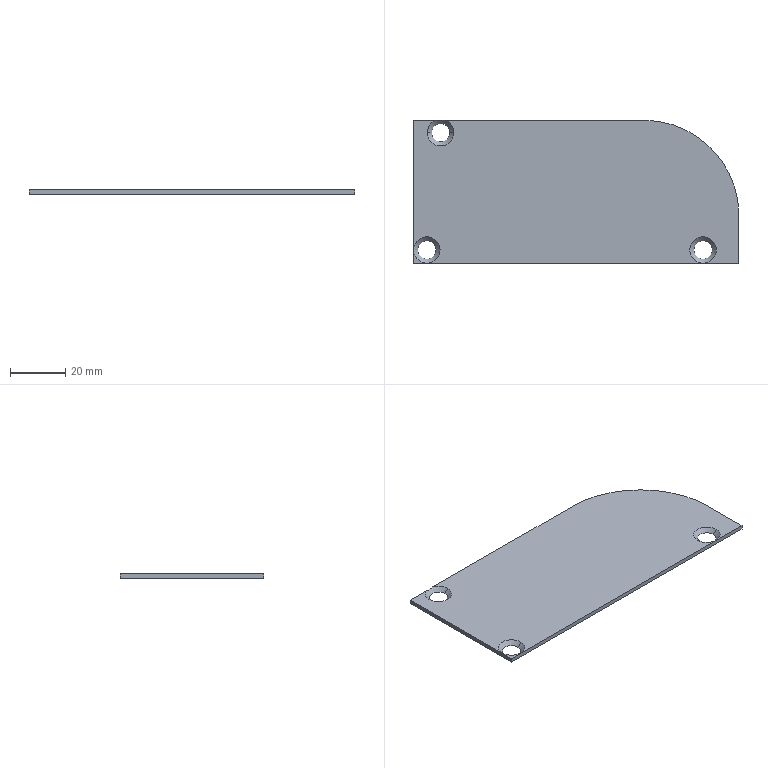Part | STEP file | 601-01-0001 | 1 solid | 13 faces | box 118 x 52 x 1.5 mm | volume 8586 mm3 | cone 6 | plane 6 | cylinder 1 | commonest cylinder face diameters 69 x1
STEP:
#1=CARTESIAN_POINT('',(0.,0.,0.));
#2=DIRECTION('',(0.,0.,1.));
#3=DIRECTION('',(1.,0.,0.));
#4=AXIS2_PLACEMENT_3D('',#1,#2,#3);
#5=CARTESIAN_POINT('',(-45.7,21.5,0.));
#6=VERTEX_POINT('',#5);
#7=CARTESIAN_POINT('',(-44.2,21.5,1.5));
#8=VERTEX_POINT('',#7);
#9=CARTESIAN_POINT('',(-44.2,21.5,1.5));
#10=DIRECTION('',(0.7071,0.,0.7071));
#11=VECTOR('',#10,1.);
#12=LINE('',#9,#11);
#13=CARTESIAN_POINT('',(-49.,21.5,1.5));
#14=DIRECTION('',(0.,0.,1.));
#15=DIRECTION('',(1.,0.,0.));
#16=AXIS2_PLACEMENT_3D('',#13,#14,#15);
#17=CONICAL_SURFACE('',#16,4.8,0.7854);
#18=CARTESIAN_POINT('',(6.283,0.));
#19=DIRECTION('',(0.,1.));
#20=VECTOR('',#19,1.);
#21=LINE('',#18,#20);
#22=(GEOMETRIC_REPRESENTATION_CONTEXT(2)PARAMETRIC_REPRESENTATION_CONTEXT()REPRESENTATION_CONTEXT('',''));
#23=DEFINITIONAL_REPRESENTATION('',(#21),#22);
#24=PCURVE('',#17,#23);
#25=CARTESIAN_POINT('',(-49.,21.5,1.5));
#26=DIRECTION('',(0.,0.,1.));
#27=DIRECTION('',(1.,0.,0.));
#28=AXIS2_PLACEMENT_3D('',#25,#26,#27);
#29=CONICAL_SURFACE('',#28,4.8,0.7854);
#30=CARTESIAN_POINT('',(0.,0.));
#31=DIRECTION('',(0.,1.));
#32=VECTOR('',#31,1.);
#33=LINE('',#30,#32);
#34=(GEOMETRIC_REPRESENTATION_CONTEXT(2)PARAMETRIC_REPRESENTATION_CONTEXT()REPRESENTATION_CONTEXT('',''));
#35=DEFINITIONAL_REPRESENTATION('',(#33),#34);
#36=PCURVE('',#29,#35);
#37=SURFACE_CURVE('',#12,(#24,#36),.PCURVE_S1.);
#38=EDGE_CURVE('',#6,#8,#37,.T.);
#39=ORIENTED_EDGE('',*,*,#38,.T.);
#40=CARTESIAN_POINT('',(-53.8,21.5,1.5));
#41=VERTEX_POINT('',#40);
#42=CARTESIAN_POINT('',(-49.,21.5,1.5));
#43=DIRECTION('',(0.,0.,1.));
#44=DIRECTION('',(1.,0.,0.));
#45=AXIS2_PLACEMENT_3D('',#42,#43,#44);
#46=CIRCLE('',#45,4.8);
#47=CARTESIAN_POINT('',(0.,0.));
#48=DIRECTION('',(1.,0.));
#49=VECTOR('',#48,1.);
#50=LINE('',#47,#49);
#51=(GEOMETRIC_REPRESENTATION_CONTEXT(2)PARAMETRIC_REPRESENTATION_CONTEXT()REPRESENTATION_CONTEXT('',''));
#52=DEFINITIONAL_REPRESENTATION('',(#50),#51);
#53=PCURVE('',#17,#52);
#54=CARTESIAN_POINT('',(59.,-26.,1.5));
#55=DIRECTION('',(0.,0.,1.));
#56=DIRECTION('',(1.,0.,0.));
#57=AXIS2_PLACEMENT_3D('',#54,#55,#56);
#58=PLANE('',#57);
#59=CARTESIAN_POINT('',(-108.,47.5));
#60=DIRECTION('',(1.,0.));
#61=AXIS2_PLACEMENT_2D('',#59,#60);
#62=CIRCLE('',#61,4.8);
#63=(GEOMETRIC_REPRESENTATION_CONTEXT(2)PARAMETRIC_REPRESENTATION_CONTEXT()REPRESENTATION_CONTEXT('',''));
#64=DEFINITIONAL_REPRESENTATION('',(#62),#63);
#65=PCURVE('',#58,#64);
#66=SURFACE_CURVE('',#46,(#53,#65),.PCURVE_S1.);
#67=EDGE_CURVE('',#41,#8,#66,.T.);
#68=ORIENTED_EDGE('',*,*,#67,.F.);
#69=CARTESIAN_POINT('',(-52.3,21.5,0.));
#70=VERTEX_POINT('',#69);
#71=CARTESIAN_POINT('',(-53.8,21.5,1.5));
#72=DIRECTION('',(-0.7071,0.,0.7071));
#73=VECTOR('',#72,1.);
#74=LINE('',#71,#73);
#75=CARTESIAN_POINT('',(3.142,0.));
#76=DIRECTION('',(0.,1.));
#77=VECTOR('',#76,1.);
#78=LINE('',#75,#77);
#79=(GEOMETRIC_REPRESENTATION_CONTEXT(2)PARAMETRIC_REPRESENTATION_CONTEXT()REPRESENTATION_CONTEXT('',''));
#80=DEFINITIONAL_REPRESENTATION('',(#78),#79);
#81=PCURVE('',#17,#80);
#82=CARTESIAN_POINT('',(3.142,0.));
#83=DIRECTION('',(0.,1.));
#84=VECTOR('',#83,1.);
#85=LINE('',#82,#84);
#86=(GEOMETRIC_REPRESENTATION_CONTEXT(2)PARAMETRIC_REPRESENTATION_CONTEXT()REPRESENTATION_CONTEXT('',''));
#87=DEFINITIONAL_REPRESENTATION('',(#85),#86);
#88=PCURVE('',#29,#87);
#89=SURFACE_CURVE('',#74,(#81,#88),.PCURVE_S1.);
#90=EDGE_CURVE('',#70,#41,#89,.T.);
#91=ORIENTED_EDGE('',*,*,#90,.F.);
#92=CARTESIAN_POINT('',(-49.,21.5,0.));
#93=DIRECTION('',(0.,0.,1.));
#94=DIRECTION('',(1.,0.,0.));
#95=AXIS2_PLACEMENT_3D('',#92,#93,#94);
#96=CIRCLE('',#95,3.3);
#97=CARTESIAN_POINT('',(0.,-1.5));
#98=DIRECTION('',(1.,0.));
#99=VECTOR('',#98,1.);
#100=LINE('',#97,#99);
#101=(GEOMETRIC_REPRESENTATION_CONTEXT(2)PARAMETRIC_REPRESENTATION_CONTEXT()REPRESENTATION_CONTEXT('',''));
#102=DEFINITIONAL_REPRESENTATION('',(#100),#101);
#103=PCURVE('',#17,#102);
#104=CARTESIAN_POINT('',(59.,-26.,0.));
#105=DIRECTION('',(0.,0.,1.));
#106=DIRECTION('',(1.,0.,0.));
#107=AXIS2_PLACEMENT_3D('',#104,#105,#106);
#108=PLANE('',#107);
#109=CARTESIAN_POINT('',(-108.,47.5));
#110=DIRECTION('',(1.,0.));
#111=AXIS2_PLACEMENT_2D('',#109,#110);
#112=CIRCLE('',#111,3.3);
#113=(GEOMETRIC_REPRESENTATION_CONTEXT(2)PARAMETRIC_REPRESENTATION_CONTEXT()REPRESENTATION_CONTEXT('',''));
#114=DEFINITIONAL_REPRESENTATION('',(#112),#113);
#115=PCURVE('',#108,#114);
#116=SURFACE_CURVE('',#96,(#103,#115),.PCURVE_S1.);
#117=EDGE_CURVE('',#70,#6,#116,.T.);
#118=ORIENTED_EDGE('',*,*,#117,.T.);
#119=EDGE_LOOP('',(#39,#68,#91,#118));
#120=FACE_BOUND('',#119,.F.);
#121=ADVANCED_FACE('',(#120),#17,.F.);
#122=CARTESIAN_POINT('',(-50.7,-21.,0.));
#123=VERTEX_POINT('',#122);
#124=CARTESIAN_POINT('',(-49.2,-21.,1.5));
#125=VERTEX_POINT('',#124);
#126=CARTESIAN_POINT('',(-49.2,-21.,1.5));
#127=DIRECTION('',(0.7071,0.,0.7071));
#128=VECTOR('',#127,1.);
#129=LINE('',#126,#128);
#130=CARTESIAN_POINT('',(-54.,-21.,1.5));
#131=DIRECTION('',(0.,0.,1.));
#132=DIRECTION('',(1.,0.,0.));
#133=AXIS2_PLACEMENT_3D('',#130,#131,#132);
#134=CONICAL_SURFACE('',#133,4.8,0.7854);
#135=CARTESIAN_POINT('',(6.283,0.));
#136=DIRECTION('',(0.,1.));
#137=VECTOR('',#136,1.);
#138=LINE('',#135,#137);
#139=(GEOMETRIC_REPRESENTATION_CONTEXT(2)PARAMETRIC_REPRESENTATION_CONTEXT()REPRESENTATION_CONTEXT('',''));
#140=DEFINITIONAL_REPRESENTATION('',(#138),#139);
#141=PCURVE('',#134,#140);
#142=CARTESIAN_POINT('',(-54.,-21.,1.5));
#143=DIRECTION('',(0.,0.,1.));
#144=DIRECTION('',(1.,0.,0.));
#145=AXIS2_PLACEMENT_3D('',#142,#143,#144);
#146=CONICAL_SURFACE('',#145,4.8,0.7854);
#147=CARTESIAN_POINT('',(0.,0.));
#148=DIRECTION('',(0.,1.));
#149=VECTOR('',#148,1.);
#150=LINE('',#147,#149);
#151=(GEOMETRIC_REPRESENTATION_CONTEXT(2)PARAMETRIC_REPRESENTATION_CONTEXT()REPRESENTATION_CONTEXT('',''));
#152=DEFINITIONAL_REPRESENTATION('',(#150),#151);
#153=PCURVE('',#146,#152);
#154=SURFACE_CURVE('',#129,(#141,#153),.PCURVE_S1.);
#155=EDGE_CURVE('',#123,#125,#154,.T.);
#156=ORIENTED_EDGE('',*,*,#155,.T.);
#157=CARTESIAN_POINT('',(-58.8,-21.,1.5));
#158=VERTEX_POINT('',#157);
#159=CARTESIAN_POINT('',(-54.,-21.,1.5));
#160=DIRECTION('',(0.,0.,1.));
#161=DIRECTION('',(1.,0.,0.));
#162=AXIS2_PLACEMENT_3D('',#159,#160,#161);
#163=CIRCLE('',#162,4.8);
#164=CARTESIAN_POINT('',(0.,0.));
#165=DIRECTION('',(1.,0.));
#166=VECTOR('',#165,1.);
#167=LINE('',#164,#166);
#168=(GEOMETRIC_REPRESENTATION_CONTEXT(2)PARAMETRIC_REPRESENTATION_CONTEXT()REPRESENTATION_CONTEXT('',''));
#169=DEFINITIONAL_REPRESENTATION('',(#167),#168);
#170=PCURVE('',#134,#169);
#171=CARTESIAN_POINT('',(-113.,5.));
#172=DIRECTION('',(1.,0.));
#173=AXIS2_PLACEMENT_2D('',#171,#172);
#174=CIRCLE('',#173,4.8);
#175=(GEOMETRIC_REPRESENTATION_CONTEXT(2)PARAMETRIC_REPRESENTATION_CONTEXT()REPRESENTATION_CONTEXT('',''));
#176=DEFINITIONAL_REPRESENTATION('',(#174),#175);
#177=PCURVE('',#58,#176);
#178=SURFACE_CURVE('',#163,(#170,#177),.PCURVE_S1.);
#179=EDGE_CURVE('',#158,#125,#178,.T.);
#180=ORIENTED_EDGE('',*,*,#179,.F.);
#181=CARTESIAN_POINT('',(-57.3,-21.,0.));
#182=VERTEX_POINT('',#181);
#183=CARTESIAN_POINT('',(-58.8,-21.,1.5));
#184=DIRECTION('',(-0.7071,0.,0.7071));
#185=VECTOR('',#184,1.);
#186=LINE('',#183,#185);
#187=CARTESIAN_POINT('',(3.142,0.));
#188=DIRECTION('',(0.,1.));
#189=VECTOR('',#188,1.);
#190=LINE('',#187,#189);
#191=(GEOMETRIC_REPRESENTATION_CONTEXT(2)PARAMETRIC_REPRESENTATION_CONTEXT()REPRESENTATION_CONTEXT('',''));
#192=DEFINITIONAL_REPRESENTATION('',(#190),#191);
#193=PCURVE('',#134,#192);
#194=CARTESIAN_POINT('',(3.142,0.));
#195=DIRECTION('',(0.,1.));
#196=VECTOR('',#195,1.);
#197=LINE('',#194,#196);
#198=(GEOMETRIC_REPRESENTATION_CONTEXT(2)PARAMETRIC_REPRESENTATION_CONTEXT()REPRESENTATION_CONTEXT('',''));
#199=DEFINITIONAL_REPRESENTATION('',(#197),#198);
#200=PCURVE('',#146,#199);
#201=SURFACE_CURVE('',#186,(#193,#200),.PCURVE_S1.);
#202=EDGE_CURVE('',#182,#158,#201,.T.);
#203=ORIENTED_EDGE('',*,*,#202,.F.);
#204=CARTESIAN_POINT('',(-54.,-21.,0.));
#205=DIRECTION('',(0.,0.,1.));
#206=DIRECTION('',(1.,0.,0.));
#207=AXIS2_PLACEMENT_3D('',#204,#205,#206);
#208=CIRCLE('',#207,3.3);
#209=CARTESIAN_POINT('',(0.,-1.5));
#210=DIRECTION('',(1.,0.));
#211=VECTOR('',#210,1.);
#212=LINE('',#209,#211);
#213=(GEOMETRIC_REPRESENTATION_CONTEXT(2)PARAMETRIC_REPRESENTATION_CONTEXT()REPRESENTATION_CONTEXT('',''));
#214=DEFINITIONAL_REPRESENTATION('',(#212),#213);
#215=PCURVE('',#134,#214);
#216=CARTESIAN_POINT('',(-113.,5.));
#217=DIRECTION('',(1.,0.));
#218=AXIS2_PLACEMENT_2D('',#216,#217);
#219=CIRCLE('',#218,3.3);
#220=(GEOMETRIC_REPRESENTATION_CONTEXT(2)PARAMETRIC_REPRESENTATION_CONTEXT()REPRESENTATION_CONTEXT('',''));
#221=DEFINITIONAL_REPRESENTATION('',(#219),#220);
#222=PCURVE('',#108,#221);
#223=SURFACE_CURVE('',#208,(#215,#222),.PCURVE_S1.);
#224=EDGE_CURVE('',#182,#123,#223,.T.);
#225=ORIENTED_EDGE('',*,*,#224,.T.);
#226=EDGE_LOOP('',(#156,#180,#203,#225));
#227=FACE_BOUND('',#226,.F.);
#228=ADVANCED_FACE('',(#227),#134,.F.);
#229=CARTESIAN_POINT('',(49.3,-21.,0.));
#230=VERTEX_POINT('',#229);
#231=CARTESIAN_POINT('',(50.8,-21.,1.5));
#232=VERTEX_POINT('',#231);
#233=CARTESIAN_POINT('',(50.8,-21.,1.5));
#234=DIRECTION('',(0.7071,0.,0.7071));
#235=VECTOR('',#234,1.);
#236=LINE('',#233,#235);
#237=CARTESIAN_POINT('',(46.,-21.,1.5));
#238=DIRECTION('',(0.,0.,1.));
#239=DIRECTION('',(1.,0.,0.));
#240=AXIS2_PLACEMENT_3D('',#237,#238,#239);
#241=CONICAL_SURFACE('',#240,4.8,0.7854);
#242=CARTESIAN_POINT('',(6.283,0.));
#243=DIRECTION('',(0.,1.));
#244=VECTOR('',#243,1.);
#245=LINE('',#242,#244);
#246=(GEOMETRIC_REPRESENTATION_CONTEXT(2)PARAMETRIC_REPRESENTATION_CONTEXT()REPRESENTATION_CONTEXT('',''));
#247=DEFINITIONAL_REPRESENTATION('',(#245),#246);
#248=PCURVE('',#241,#247);
#249=CARTESIAN_POINT('',(46.,-21.,1.5));
#250=DIRECTION('',(0.,0.,1.));
#251=DIRECTION('',(1.,0.,0.));
#252=AXIS2_PLACEMENT_3D('',#249,#250,#251);
#253=CONICAL_SURFACE('',#252,4.8,0.7854);
#254=CARTESIAN_POINT('',(0.,0.));
#255=DIRECTION('',(0.,1.));
#256=VECTOR('',#255,1.);
#257=LINE('',#254,#256);
#258=(GEOMETRIC_REPRESENTATION_CONTEXT(2)PARAMETRIC_REPRESENTATION_CONTEXT()REPRESENTATION_CONTEXT('',''));
#259=DEFINITIONAL_REPRESENTATION('',(#257),#258);
#260=PCURVE('',#253,#259);
#261=SURFACE_CURVE('',#236,(#248,#260),.PCURVE_S1.);
#262=EDGE_CURVE('',#230,#232,#261,.T.);
#263=ORIENTED_EDGE('',*,*,#262,.T.);
#264=CARTESIAN_POINT('',(41.2,-21.,1.5));
#265=VERTEX_POINT('',#264);
#266=CARTESIAN_POINT('',(46.,-21.,1.5));
#267=DIRECTION('',(0.,0.,1.));
#268=DIRECTION('',(1.,0.,0.));
#269=AXIS2_PLACEMENT_3D('',#266,#267,#268);
#270=CIRCLE('',#269,4.8);
#271=CARTESIAN_POINT('',(0.,0.));
#272=DIRECTION('',(1.,0.));
#273=VECTOR('',#272,1.);
#274=LINE('',#271,#273);
#275=(GEOMETRIC_REPRESENTATION_CONTEXT(2)PARAMETRIC_REPRESENTATION_CONTEXT()REPRESENTATION_CONTEXT('',''));
#276=DEFINITIONAL_REPRESENTATION('',(#274),#275);
#277=PCURVE('',#241,#276);
#278=CARTESIAN_POINT('',(-13.,5.));
#279=DIRECTION('',(1.,0.));
#280=AXIS2_PLACEMENT_2D('',#278,#279);
#281=CIRCLE('',#280,4.8);
#282=(GEOMETRIC_REPRESENTATION_CONTEXT(2)PARAMETRIC_REPRESENTATION_CONTEXT()REPRESENTATION_CONTEXT('',''));
#283=DEFINITIONAL_REPRESENTATION('',(#281),#282);
#284=PCURVE('',#58,#283);
#285=SURFACE_CURVE('',#270,(#277,#284),.PCURVE_S1.);
#286=EDGE_CURVE('',#265,#232,#285,.T.);
#287=ORIENTED_EDGE('',*,*,#286,.F.);
#288=CARTESIAN_POINT('',(42.7,-21.,0.));
#289=VERTEX_POINT('',#288);
#290=CARTESIAN_POINT('',(41.2,-21.,1.5));
#291=DIRECTION('',(-0.7071,0.,0.7071));
#292=VECTOR('',#291,1.);
#293=LINE('',#290,#292);
#294=CARTESIAN_POINT('',(3.142,0.));
#295=DIRECTION('',(0.,1.));
#296=VECTOR('',#295,1.);
#297=LINE('',#294,#296);
#298=(GEOMETRIC_REPRESENTATION_CONTEXT(2)PARAMETRIC_REPRESENTATION_CONTEXT()REPRESENTATION_CONTEXT('',''));
#299=DEFINITIONAL_REPRESENTATION('',(#297),#298);
#300=PCURVE('',#241,#299);
#301=CARTESIAN_POINT('',(3.142,0.));
#302=DIRECTION('',(0.,1.));
#303=VECTOR('',#302,1.);
#304=LINE('',#301,#303);
#305=(GEOMETRIC_REPRESENTATION_CONTEXT(2)PARAMETRIC_REPRESENTATION_CONTEXT()REPRESENTATION_CONTEXT('',''));
#306=DEFINITIONAL_REPRESENTATION('',(#304),#305);
#307=PCURVE('',#253,#306);
#308=SURFACE_CURVE('',#293,(#300,#307),.PCURVE_S1.);
#309=EDGE_CURVE('',#289,#265,#308,.T.);
#310=ORIENTED_EDGE('',*,*,#309,.F.);
#311=CARTESIAN_POINT('',(46.,-21.,0.));
#312=DIRECTION('',(0.,0.,1.));
#313=DIRECTION('',(1.,0.,0.));
#314=AXIS2_PLACEMENT_3D('',#311,#312,#313);
#315=CIRCLE('',#314,3.3);
#316=CARTESIAN_POINT('',(0.,-1.5));
#317=DIRECTION('',(1.,0.));
#318=VECTOR('',#317,1.);
#319=LINE('',#316,#318);
#320=(GEOMETRIC_REPRESENTATION_CONTEXT(2)PARAMETRIC_REPRESENTATION_CONTEXT()REPRESENTATION_CONTEXT('',''));
#321=DEFINITIONAL_REPRESENTATION('',(#319),#320);
#322=PCURVE('',#241,#321);
#323=CARTESIAN_POINT('',(-13.,5.));
#324=DIRECTION('',(1.,0.));
#325=AXIS2_PLACEMENT_2D('',#323,#324);
#326=CIRCLE('',#325,3.3);
#327=(GEOMETRIC_REPRESENTATION_CONTEXT(2)PARAMETRIC_REPRESENTATION_CONTEXT()REPRESENTATION_CONTEXT('',''));
#328=DEFINITIONAL_REPRESENTATION('',(#326),#327);
#329=PCURVE('',#108,#328);
#330=SURFACE_CURVE('',#315,(#322,#329),.PCURVE_S1.);
#331=EDGE_CURVE('',#289,#230,#330,.T.);
#332=ORIENTED_EDGE('',*,*,#331,.T.);
#333=EDGE_LOOP('',(#263,#287,#310,#332));
#334=FACE_BOUND('',#333,.F.);
#335=ADVANCED_FACE('',(#334),#241,.F.);
#336=CARTESIAN_POINT('',(-49.,21.5,0.));
#337=DIRECTION('',(0.,0.,1.));
#338=DIRECTION('',(1.,0.,0.));
#339=AXIS2_PLACEMENT_3D('',#336,#337,#338);
#340=CIRCLE('',#339,3.3);
#341=CARTESIAN_POINT('',(-108.,47.5));
#342=DIRECTION('',(1.,0.));
#343=AXIS2_PLACEMENT_2D('',#341,#342);
#344=CIRCLE('',#343,3.3);
#345=(GEOMETRIC_REPRESENTATION_CONTEXT(2)PARAMETRIC_REPRESENTATION_CONTEXT()REPRESENTATION_CONTEXT('',''));
#346=DEFINITIONAL_REPRESENTATION('',(#344),#345);
#347=PCURVE('',#108,#346);
#348=CARTESIAN_POINT('',(0.,-1.5));
#349=DIRECTION('',(1.,0.));
#350=VECTOR('',#349,1.);
#351=LINE('',#348,#350);
#352=(GEOMETRIC_REPRESENTATION_CONTEXT(2)PARAMETRIC_REPRESENTATION_CONTEXT()REPRESENTATION_CONTEXT('',''));
#353=DEFINITIONAL_REPRESENTATION('',(#351),#352);
#354=PCURVE('',#29,#353);
#355=SURFACE_CURVE('',#340,(#347,#354),.PCURVE_S1.);
#356=EDGE_CURVE('',#6,#70,#355,.T.);
#357=ORIENTED_EDGE('',*,*,#356,.T.);
#358=ORIENTED_EDGE('',*,*,#117,.T.);
#359=EDGE_LOOP('',(#357,#358));
#360=FACE_BOUND('',#359,.T.);
#361=CARTESIAN_POINT('',(-54.,-21.,0.));
#362=DIRECTION('',(0.,0.,1.));
#363=DIRECTION('',(1.,0.,0.));
#364=AXIS2_PLACEMENT_3D('',#361,#362,#363);
#365=CIRCLE('',#364,3.3);
#366=CARTESIAN_POINT('',(-113.,5.));
#367=DIRECTION('',(1.,0.));
#368=AXIS2_PLACEMENT_2D('',#366,#367);
#369=CIRCLE('',#368,3.3);
#370=(GEOMETRIC_REPRESENTATION_CONTEXT(2)PARAMETRIC_REPRESENTATION_CONTEXT()REPRESENTATION_CONTEXT('',''));
#371=DEFINITIONAL_REPRESENTATION('',(#369),#370);
#372=PCURVE('',#108,#371);
#373=CARTESIAN_POINT('',(0.,-1.5));
#374=DIRECTION('',(1.,0.));
#375=VECTOR('',#374,1.);
#376=LINE('',#373,#375);
#377=(GEOMETRIC_REPRESENTATION_CONTEXT(2)PARAMETRIC_REPRESENTATION_CONTEXT()REPRESENTATION_CONTEXT('',''));
#378=DEFINITIONAL_REPRESENTATION('',(#376),#377);
#379=PCURVE('',#146,#378);
#380=SURFACE_CURVE('',#365,(#372,#379),.PCURVE_S1.);
#381=EDGE_CURVE('',#123,#182,#380,.T.);
#382=ORIENTED_EDGE('',*,*,#381,.T.);
#383=ORIENTED_EDGE('',*,*,#224,.T.);
#384=EDGE_LOOP('',(#382,#383));
#385=FACE_BOUND('',#384,.T.);
#386=CARTESIAN_POINT('',(24.5,26.,0.));
#387=VERTEX_POINT('',#386);
#388=CARTESIAN_POINT('',(-59.,26.,0.));
#389=VERTEX_POINT('',#388);
#390=CARTESIAN_POINT('',(-59.,26.,0.));
#391=DIRECTION('',(-1.,0.,0.));
#392=VECTOR('',#391,1.);
#393=LINE('',#390,#392);
#394=CARTESIAN_POINT('',(-118.,52.));
#395=DIRECTION('',(-1.,0.));
#396=VECTOR('',#395,1.);
#397=LINE('',#394,#396);
#398=(GEOMETRIC_REPRESENTATION_CONTEXT(2)PARAMETRIC_REPRESENTATION_CONTEXT()REPRESENTATION_CONTEXT('',''));
#399=DEFINITIONAL_REPRESENTATION('',(#397),#398);
#400=PCURVE('',#108,#399);
#401=CARTESIAN_POINT('',(-59.,26.,1.5));
#402=DIRECTION('',(0.,-1.,0.));
#403=DIRECTION('',(0.,0.,-1.));
#404=AXIS2_PLACEMENT_3D('',#401,#402,#403);
#405=PLANE('',#404);
#406=CARTESIAN_POINT('',(1.5,0.));
#407=DIRECTION('',(0.,-1.));
#408=VECTOR('',#407,1.);
#409=LINE('',#406,#408);
#410=(GEOMETRIC_REPRESENTATION_CONTEXT(2)PARAMETRIC_REPRESENTATION_CONTEXT()REPRESENTATION_CONTEXT('',''));
#411=DEFINITIONAL_REPRESENTATION('',(#409),#410);
#412=PCURVE('',#405,#411);
#413=SURFACE_CURVE('',#393,(#400,#412),.PCURVE_S1.);
#414=EDGE_CURVE('',#387,#389,#413,.T.);
#415=ORIENTED_EDGE('',*,*,#414,.F.);
#416=CARTESIAN_POINT('',(59.,-8.5,0.));
#417=VERTEX_POINT('',#416);
#418=CARTESIAN_POINT('',(24.5,-8.5,0.));
#419=DIRECTION('',(0.,0.,-1.));
#420=DIRECTION('',(1.,0.,0.));
#421=AXIS2_PLACEMENT_3D('',#418,#419,#420);
#422=CIRCLE('',#421,34.5);
#423=CARTESIAN_POINT('',(0.,17.5));
#424=CARTESIAN_POINT('',(0.,-42.256));
#425=CARTESIAN_POINT('',(-51.75,-12.378));
#426=CARTESIAN_POINT('',(-103.5,17.5));
#427=CARTESIAN_POINT('',(-51.75,47.378));
#428=CARTESIAN_POINT('',(0.,77.256));
#429=CARTESIAN_POINT('',(0.,17.5));
#430=(BOUNDED_CURVE()B_SPLINE_CURVE(2,(#423,#424,#425,#426,#427,#428,#429),.UNSPECIFIED.,.T.,.F.)B_SPLINE_CURVE_WITH_KNOTS((1,2,2,2,2,1),(-2.094,0.,2.094,4.189,6.283,8.378),.UNSPECIFIED.)CURVE()GEOMETRIC_REPRESENTATION_ITEM()RATIONAL_B_SPLINE_CURVE((1.,0.5,1.,0.5,1.,0.5,1.))REPRESENTATION_ITEM(''));
#431=(GEOMETRIC_REPRESENTATION_CONTEXT(2)PARAMETRIC_REPRESENTATION_CONTEXT()REPRESENTATION_CONTEXT('',''));
#432=DEFINITIONAL_REPRESENTATION('',(#430),#431);
#433=PCURVE('',#108,#432);
#434=CARTESIAN_POINT('',(24.5,-8.5,1.5));
#435=DIRECTION('',(0.,0.,-1.));
#436=DIRECTION('',(-1.,0.,0.));
#437=AXIS2_PLACEMENT_3D('',#434,#435,#436);
#438=CYLINDRICAL_SURFACE('',#437,34.5);
#439=CARTESIAN_POINT('',(-3.142,1.5));
#440=DIRECTION('',(1.,0.));
#441=VECTOR('',#440,1.);
#442=LINE('',#439,#441);
#443=(GEOMETRIC_REPRESENTATION_CONTEXT(2)PARAMETRIC_REPRESENTATION_CONTEXT()REPRESENTATION_CONTEXT('',''));
#444=DEFINITIONAL_REPRESENTATION('',(#442),#443);
#445=PCURVE('',#438,#444);
#446=SURFACE_CURVE('',#422,(#433,#445),.PCURVE_S1.);
#447=EDGE_CURVE('',#387,#417,#446,.T.);
#448=ORIENTED_EDGE('',*,*,#447,.T.);
#449=CARTESIAN_POINT('',(59.,-26.,0.));
#450=VERTEX_POINT('',#449);
#451=CARTESIAN_POINT('',(59.,26.,0.));
#452=DIRECTION('',(0.,1.,0.));
#453=VECTOR('',#452,1.);
#454=LINE('',#451,#453);
#455=CARTESIAN_POINT('',(0.,52.));
#456=DIRECTION('',(0.,1.));
#457=VECTOR('',#456,1.);
#458=LINE('',#455,#457);
#459=(GEOMETRIC_REPRESENTATION_CONTEXT(2)PARAMETRIC_REPRESENTATION_CONTEXT()REPRESENTATION_CONTEXT('',''));
#460=DEFINITIONAL_REPRESENTATION('',(#458),#459);
#461=PCURVE('',#108,#460);
#462=CARTESIAN_POINT('',(59.,26.,1.5));
#463=DIRECTION('',(-1.,0.,0.));
#464=DIRECTION('',(0.,-1.,0.));
#465=AXIS2_PLACEMENT_3D('',#462,#463,#464);
#466=PLANE('',#465);
#467=CARTESIAN_POINT('',(0.,-1.5));
#468=DIRECTION('',(-1.,0.));
#469=VECTOR('',#468,1.);
#470=LINE('',#467,#469);
#471=(GEOMETRIC_REPRESENTATION_CONTEXT(2)PARAMETRIC_REPRESENTATION_CONTEXT()REPRESENTATION_CONTEXT('',''));
#472=DEFINITIONAL_REPRESENTATION('',(#470),#471);
#473=PCURVE('',#466,#472);
#474=SURFACE_CURVE('',#454,(#461,#473),.PCURVE_S1.);
#475=EDGE_CURVE('',#450,#417,#474,.T.);
#476=ORIENTED_EDGE('',*,*,#475,.F.);
#477=CARTESIAN_POINT('',(-59.,-26.,0.));
#478=VERTEX_POINT('',#477);
#479=CARTESIAN_POINT('',(-59.,-26.,0.));
#480=DIRECTION('',(1.,0.,0.));
#481=VECTOR('',#480,1.);
#482=LINE('',#479,#481);
#483=CARTESIAN_POINT('',(-118.,0.));
#484=DIRECTION('',(1.,0.));
#485=VECTOR('',#484,1.);
#486=LINE('',#483,#485);
#487=(GEOMETRIC_REPRESENTATION_CONTEXT(2)PARAMETRIC_REPRESENTATION_CONTEXT()REPRESENTATION_CONTEXT('',''));
#488=DEFINITIONAL_REPRESENTATION('',(#486),#487);
#489=PCURVE('',#108,#488);
#490=CARTESIAN_POINT('',(-59.,-26.,1.5));
#491=DIRECTION('',(0.,1.,0.));
#492=DIRECTION('',(0.,0.,1.));
#493=AXIS2_PLACEMENT_3D('',#490,#491,#492);
#494=PLANE('',#493);
#495=CARTESIAN_POINT('',(-1.5,0.));
#496=DIRECTION('',(0.,1.));
#497=VECTOR('',#496,1.);
#498=LINE('',#495,#497);
#499=(GEOMETRIC_REPRESENTATION_CONTEXT(2)PARAMETRIC_REPRESENTATION_CONTEXT()REPRESENTATION_CONTEXT('',''));
#500=DEFINITIONAL_REPRESENTATION('',(#498),#499);
#501=PCURVE('',#494,#500);
#502=SURFACE_CURVE('',#482,(#489,#501),.PCURVE_S1.);
#503=EDGE_CURVE('',#478,#450,#502,.T.);
#504=ORIENTED_EDGE('',*,*,#503,.F.);
#505=CARTESIAN_POINT('',(-59.,26.,0.));
#506=DIRECTION('',(0.,-1.,0.));
#507=VECTOR('',#506,1.);
#508=LINE('',#505,#507);
#509=CARTESIAN_POINT('',(-118.,52.));
#510=DIRECTION('',(0.,-1.));
#511=VECTOR('',#510,1.);
#512=LINE('',#509,#511);
#513=(GEOMETRIC_REPRESENTATION_CONTEXT(2)PARAMETRIC_REPRESENTATION_CONTEXT()REPRESENTATION_CONTEXT('',''));
#514=DEFINITIONAL_REPRESENTATION('',(#512),#513);
#515=PCURVE('',#108,#514);
#516=CARTESIAN_POINT('',(-59.,26.,1.5));
#517=DIRECTION('',(1.,0.,0.));
#518=DIRECTION('',(0.,1.,0.));
#519=AXIS2_PLACEMENT_3D('',#516,#517,#518);
#520=PLANE('',#519);
#521=CARTESIAN_POINT('',(0.,-1.5));
#522=DIRECTION('',(-1.,0.));
#523=VECTOR('',#522,1.);
#524=LINE('',#521,#523);
#525=(GEOMETRIC_REPRESENTATION_CONTEXT(2)PARAMETRIC_REPRESENTATION_CONTEXT()REPRESENTATION_CONTEXT('',''));
#526=DEFINITIONAL_REPRESENTATION('',(#524),#525);
#527=PCURVE('',#520,#526);
#528=SURFACE_CURVE('',#508,(#515,#527),.PCURVE_S1.);
#529=EDGE_CURVE('',#389,#478,#528,.T.);
#530=ORIENTED_EDGE('',*,*,#529,.F.);
#531=EDGE_LOOP('',(#415,#448,#476,#504,#530));
#532=FACE_BOUND('',#531,.T.);
#533=CARTESIAN_POINT('',(46.,-21.,0.));
#534=DIRECTION('',(0.,0.,1.));
#535=DIRECTION('',(1.,0.,0.));
#536=AXIS2_PLACEMENT_3D('',#533,#534,#535);
#537=CIRCLE('',#536,3.3);
#538=CARTESIAN_POINT('',(-13.,5.));
#539=DIRECTION('',(1.,0.));
#540=AXIS2_PLACEMENT_2D('',#538,#539);
#541=CIRCLE('',#540,3.3);
#542=(GEOMETRIC_REPRESENTATION_CONTEXT(2)PARAMETRIC_REPRESENTATION_CONTEXT()REPRESENTATION_CONTEXT('',''));
#543=DEFINITIONAL_REPRESENTATION('',(#541),#542);
#544=PCURVE('',#108,#543);
#545=CARTESIAN_POINT('',(0.,-1.5));
#546=DIRECTION('',(1.,0.));
#547=VECTOR('',#546,1.);
#548=LINE('',#545,#547);
#549=(GEOMETRIC_REPRESENTATION_CONTEXT(2)PARAMETRIC_REPRESENTATION_CONTEXT()REPRESENTATION_CONTEXT('',''));
#550=DEFINITIONAL_REPRESENTATION('',(#548),#549);
#551=PCURVE('',#253,#550);
#552=SURFACE_CURVE('',#537,(#544,#551),.PCURVE_S1.);
#553=EDGE_CURVE('',#230,#289,#552,.T.);
#554=ORIENTED_EDGE('',*,*,#553,.T.);
#555=ORIENTED_EDGE('',*,*,#331,.T.);
#556=EDGE_LOOP('',(#554,#555));
#557=FACE_BOUND('',#556,.T.);
#558=ADVANCED_FACE('',(#360,#385,#532,#557),#108,.F.);
#559=ORIENTED_EDGE('',*,*,#475,.T.);
#560=CARTESIAN_POINT('',(59.,-8.5,1.5));
#561=VERTEX_POINT('',#560);
#562=CARTESIAN_POINT('',(59.,-8.5,1.5));
#563=DIRECTION('',(0.,0.,1.));
#564=VECTOR('',#563,1.);
#565=LINE('',#562,#564);
#566=CARTESIAN_POINT('',(34.5,0.));
#567=DIRECTION('',(0.,1.));
#568=VECTOR('',#567,1.);
#569=LINE('',#566,#568);
#570=(GEOMETRIC_REPRESENTATION_CONTEXT(2)PARAMETRIC_REPRESENTATION_CONTEXT()REPRESENTATION_CONTEXT('',''));
#571=DEFINITIONAL_REPRESENTATION('',(#569),#570);
#572=PCURVE('',#466,#571);
#573=CARTESIAN_POINT('',(3.142,0.));
#574=DIRECTION('',(0.,-1.));
#575=VECTOR('',#574,1.);
#576=LINE('',#573,#575);
#577=(GEOMETRIC_REPRESENTATION_CONTEXT(2)PARAMETRIC_REPRESENTATION_CONTEXT()REPRESENTATION_CONTEXT('',''));
#578=DEFINITIONAL_REPRESENTATION('',(#576),#577);
#579=PCURVE('',#438,#578);
#580=SURFACE_CURVE('',#565,(#572,#579),.PCURVE_S1.);
#581=EDGE_CURVE('',#417,#561,#580,.T.);
#582=ORIENTED_EDGE('',*,*,#581,.T.);
#583=CARTESIAN_POINT('',(59.,-26.,1.5));
#584=VERTEX_POINT('',#583);
#585=CARTESIAN_POINT('',(59.,26.,1.5));
#586=DIRECTION('',(0.,1.,0.));
#587=VECTOR('',#586,1.);
#588=LINE('',#585,#587);
#589=CARTESIAN_POINT('',(0.,0.));
#590=DIRECTION('',(-1.,0.));
#591=VECTOR('',#590,1.);
#592=LINE('',#589,#591);
#593=(GEOMETRIC_REPRESENTATION_CONTEXT(2)PARAMETRIC_REPRESENTATION_CONTEXT()REPRESENTATION_CONTEXT('',''));
#594=DEFINITIONAL_REPRESENTATION('',(#592),#593);
#595=PCURVE('',#466,#594);
#596=CARTESIAN_POINT('',(0.,52.));
#597=DIRECTION('',(0.,1.));
#598=VECTOR('',#597,1.);
#599=LINE('',#596,#598);
#600=(GEOMETRIC_REPRESENTATION_CONTEXT(2)PARAMETRIC_REPRESENTATION_CONTEXT()REPRESENTATION_CONTEXT('',''));
#601=DEFINITIONAL_REPRESENTATION('',(#599),#600);
#602=PCURVE('',#58,#601);
#603=SURFACE_CURVE('',#588,(#595,#602),.PCURVE_S1.);
#604=EDGE_CURVE('',#584,#561,#603,.T.);
#605=ORIENTED_EDGE('',*,*,#604,.F.);
#606=CARTESIAN_POINT('',(59.,-26.,1.5));
#607=DIRECTION('',(0.,0.,-1.));
#608=VECTOR('',#607,1.);
#609=LINE('',#606,#608);
#610=CARTESIAN_POINT('',(52.,0.));
#611=DIRECTION('',(0.,-1.));
#612=VECTOR('',#611,1.);
#613=LINE('',#610,#612);
#614=(GEOMETRIC_REPRESENTATION_CONTEXT(2)PARAMETRIC_REPRESENTATION_CONTEXT()REPRESENTATION_CONTEXT('',''));
#615=DEFINITIONAL_REPRESENTATION('',(#613),#614);
#616=PCURVE('',#466,#615);
#617=CARTESIAN_POINT('',(0.,118.));
#618=DIRECTION('',(-1.,0.));
#619=VECTOR('',#618,1.);
#620=LINE('',#617,#619);
#621=(GEOMETRIC_REPRESENTATION_CONTEXT(2)PARAMETRIC_REPRESENTATION_CONTEXT()REPRESENTATION_CONTEXT('',''));
#622=DEFINITIONAL_REPRESENTATION('',(#620),#621);
#623=PCURVE('',#494,#622);
#624=SURFACE_CURVE('',#609,(#616,#623),.PCURVE_S1.);
#625=EDGE_CURVE('',#584,#450,#624,.T.);
#626=ORIENTED_EDGE('',*,*,#625,.T.);
#627=EDGE_LOOP('',(#559,#582,#605,#626));
#628=FACE_BOUND('',#627,.T.);
#629=ADVANCED_FACE('',(#628),#466,.F.);
#630=CARTESIAN_POINT('',(-50.67,26.,1.5));
#631=VERTEX_POINT('',#630);
#632=CARTESIAN_POINT('',(-59.,26.,1.5));
#633=VERTEX_POINT('',#632);
#634=CARTESIAN_POINT('',(-59.,26.,1.5));
#635=DIRECTION('',(-1.,0.,0.));
#636=VECTOR('',#635,1.);
#637=LINE('',#634,#636);
#638=CARTESIAN_POINT('',(0.,0.));
#639=DIRECTION('',(0.,-1.));
#640=VECTOR('',#639,1.);
#641=LINE('',#638,#640);
#642=(GEOMETRIC_REPRESENTATION_CONTEXT(2)PARAMETRIC_REPRESENTATION_CONTEXT()REPRESENTATION_CONTEXT('',''));
#643=DEFINITIONAL_REPRESENTATION('',(#641),#642);
#644=PCURVE('',#405,#643);
#645=CARTESIAN_POINT('',(-118.,52.));
#646=DIRECTION('',(-1.,0.));
#647=VECTOR('',#646,1.);
#648=LINE('',#645,#647);
#649=(GEOMETRIC_REPRESENTATION_CONTEXT(2)PARAMETRIC_REPRESENTATION_CONTEXT()REPRESENTATION_CONTEXT('',''));
#650=DEFINITIONAL_REPRESENTATION('',(#648),#649);
#651=PCURVE('',#58,#650);
#652=SURFACE_CURVE('',#637,(#644,#651),.PCURVE_S1.);
#653=EDGE_CURVE('',#631,#633,#652,.T.);
#654=ORIENTED_EDGE('',*,*,#653,.F.);
#655=CARTESIAN_POINT('',(-47.33,26.,1.5));
#656=VERTEX_POINT('',#655);
#657=CARTESIAN_POINT('',(-50.67,26.,1.5));
#658=CARTESIAN_POINT('',(-50.401,26.,1.406));
#659=CARTESIAN_POINT('',(-50.125,26.,1.33));
#660=CARTESIAN_POINT('',(-49.567,26.,1.227));
#661=CARTESIAN_POINT('',(-49.281,26.,1.2));
#662=CARTESIAN_POINT('',(-48.711,26.,1.2));
#663=CARTESIAN_POINT('',(-48.429,26.,1.228));
#664=CARTESIAN_POINT('',(-47.874,26.,1.331));
#665=CARTESIAN_POINT('',(-47.599,26.,1.406));
#666=CARTESIAN_POINT('',(-47.33,26.,1.5));
#667=B_SPLINE_CURVE_WITH_KNOTS('',3,(#657,#658,#659,#660,#661,#662,#663,#664,#665,#666),.UNSPECIFIED.,.F.,.F.,(4,2,2,2,4),(0.003213,0.004058,0.004902,0.005746,0.006591),.UNSPECIFIED.);
#668=CARTESIAN_POINT('',(0.,8.33));
#669=CARTESIAN_POINT('',(0.09372,8.599));
#670=CARTESIAN_POINT('',(0.1697,8.875));
#671=CARTESIAN_POINT('',(0.2728,9.433));
#672=CARTESIAN_POINT('',(0.3003,9.719));
#673=CARTESIAN_POINT('',(0.2997,10.289));
#674=CARTESIAN_POINT('',(0.2722,10.571));
#675=CARTESIAN_POINT('',(0.1694,11.126));
#676=CARTESIAN_POINT('',(0.0936,11.401));
#677=CARTESIAN_POINT('',(0.,11.67));
#678=B_SPLINE_CURVE_WITH_KNOTS('',3,(#668,#669,#670,#671,#672,#673,#674,#675,#676,#677),.UNSPECIFIED.,.F.,.F.,(4,2,2,2,4),(0.003213,0.004058,0.004902,0.005746,0.006591),.UNSPECIFIED.);
#679=(GEOMETRIC_REPRESENTATION_CONTEXT(2)PARAMETRIC_REPRESENTATION_CONTEXT()REPRESENTATION_CONTEXT('',''));
#680=DEFINITIONAL_REPRESENTATION('',(#678),#679);
#681=PCURVE('',#405,#680);
#682=CARTESIAN_POINT('',(1.926,0.));
#683=CARTESIAN_POINT('',(1.917,-0.01704));
#684=CARTESIAN_POINT('',(1.897,-0.04995));
#685=CARTESIAN_POINT('',(1.867,-0.09556));
#686=CARTESIAN_POINT('',(1.837,-0.1371));
#687=CARTESIAN_POINT('',(1.805,-0.1745));
#688=CARTESIAN_POINT('',(1.773,-0.2073));
#689=CARTESIAN_POINT('',(1.74,-0.2355));
#690=CARTESIAN_POINT('',(1.707,-0.2588));
#691=CARTESIAN_POINT('',(1.673,-0.2772));
#692=CARTESIAN_POINT('',(1.639,-0.2904));
#693=CARTESIAN_POINT('',(1.604,-0.2983));
#694=CARTESIAN_POINT('',(1.57,-0.3009));
#695=CARTESIAN_POINT('',(1.535,-0.298));
#696=CARTESIAN_POINT('',(1.501,-0.2899));
#697=CARTESIAN_POINT('',(1.467,-0.2766));
#698=CARTESIAN_POINT('',(1.434,-0.2583));
#699=CARTESIAN_POINT('',(1.401,-0.235));
#700=CARTESIAN_POINT('',(1.368,-0.2069));
#701=CARTESIAN_POINT('',(1.336,-0.1742));
#702=CARTESIAN_POINT('',(1.305,-0.1369));
#703=CARTESIAN_POINT('',(1.274,-0.09541));
#704=CARTESIAN_POINT('',(1.244,-0.04988));
#705=CARTESIAN_POINT('',(1.225,-0.01702));
#706=CARTESIAN_POINT('',(1.215,0.));
#707=B_SPLINE_CURVE_WITH_KNOTS('',3,(#682,#683,#684,#685,#686,#687,#688,#689,#690,#691,#692,#693,#694,#695,#696,#697,#698,#699,#700,#701,#702,#703,#704,#705,#706),.UNSPECIFIED.,.F.,.F.,(4,1,1,1,1,1,1,1,1,1,1,1,1,1,1,1,1,1,1,1,1,1,4),(0.003213,0.003367,0.00352,0.003674,0.003827,0.003981,0.004134,0.004288,0.004441,0.004595,0.004749,0.004902,0.005056,0.005209,0.005363,0.005516,0.00567,0.005823,0.005977,0.00613,0.006284,0.006437,0.006591),.QUASI_UNIFORM_KNOTS.);
#708=(GEOMETRIC_REPRESENTATION_CONTEXT(2)PARAMETRIC_REPRESENTATION_CONTEXT()REPRESENTATION_CONTEXT('',''));
#709=DEFINITIONAL_REPRESENTATION('',(#707),#708);
#710=PCURVE('',#29,#709);
#711=SURFACE_CURVE('',#667,(#681,#710),.PCURVE_S1.);
#712=EDGE_CURVE('',#631,#656,#711,.T.);
#713=ORIENTED_EDGE('',*,*,#712,.T.);
#714=CARTESIAN_POINT('',(24.5,26.,1.5));
#715=VERTEX_POINT('',#714);
#716=CARTESIAN_POINT('',(-59.,26.,1.5));
#717=DIRECTION('',(-1.,0.,0.));
#718=VECTOR('',#717,1.);
#719=LINE('',#716,#718);
#720=CARTESIAN_POINT('',(0.,0.));
#721=DIRECTION('',(0.,-1.));
#722=VECTOR('',#721,1.);
#723=LINE('',#720,#722);
#724=(GEOMETRIC_REPRESENTATION_CONTEXT(2)PARAMETRIC_REPRESENTATION_CONTEXT()REPRESENTATION_CONTEXT('',''));
#725=DEFINITIONAL_REPRESENTATION('',(#723),#724);
#726=PCURVE('',#405,#725);
#727=CARTESIAN_POINT('',(-118.,52.));
#728=DIRECTION('',(-1.,0.));
#729=VECTOR('',#728,1.);
#730=LINE('',#727,#729);
#731=(GEOMETRIC_REPRESENTATION_CONTEXT(2)PARAMETRIC_REPRESENTATION_CONTEXT()REPRESENTATION_CONTEXT('',''));
#732=DEFINITIONAL_REPRESENTATION('',(#730),#731);
#733=PCURVE('',#58,#732);
#734=SURFACE_CURVE('',#719,(#726,#733),.PCURVE_S1.);
#735=EDGE_CURVE('',#715,#656,#734,.T.);
#736=ORIENTED_EDGE('',*,*,#735,.F.);
#737=CARTESIAN_POINT('',(24.5,26.,1.5));
#738=DIRECTION('',(0.,0.,-1.));
#739=VECTOR('',#738,1.);
#740=LINE('',#737,#739);
#741=CARTESIAN_POINT('',(0.,83.5));
#742=DIRECTION('',(1.,0.));
#743=VECTOR('',#742,1.);
#744=LINE('',#741,#743);
#745=(GEOMETRIC_REPRESENTATION_CONTEXT(2)PARAMETRIC_REPRESENTATION_CONTEXT()REPRESENTATION_CONTEXT('',''));
#746=DEFINITIONAL_REPRESENTATION('',(#744),#745);
#747=PCURVE('',#405,#746);
#748=CARTESIAN_POINT('',(1.571,0.));
#749=DIRECTION('',(0.,1.));
#750=VECTOR('',#749,1.);
#751=LINE('',#748,#750);
#752=(GEOMETRIC_REPRESENTATION_CONTEXT(2)PARAMETRIC_REPRESENTATION_CONTEXT()REPRESENTATION_CONTEXT('',''));
#753=DEFINITIONAL_REPRESENTATION('',(#751),#752);
#754=PCURVE('',#438,#753);
#755=SURFACE_CURVE('',#740,(#747,#754),.PCURVE_S1.);
#756=EDGE_CURVE('',#715,#387,#755,.T.);
#757=ORIENTED_EDGE('',*,*,#756,.T.);
#758=ORIENTED_EDGE('',*,*,#414,.T.);
#759=CARTESIAN_POINT('',(-59.,26.,1.5));
#760=DIRECTION('',(0.,0.,-1.));
#761=VECTOR('',#760,1.);
#762=LINE('',#759,#761);
#763=CARTESIAN_POINT('',(0.,0.));
#764=DIRECTION('',(1.,0.));
#765=VECTOR('',#764,1.);
#766=LINE('',#763,#765);
#767=(GEOMETRIC_REPRESENTATION_CONTEXT(2)PARAMETRIC_REPRESENTATION_CONTEXT()REPRESENTATION_CONTEXT('',''));
#768=DEFINITIONAL_REPRESENTATION('',(#766),#767);
#769=PCURVE('',#405,#768);
#770=CARTESIAN_POINT('',(0.,0.));
#771=DIRECTION('',(0.,-1.));
#772=VECTOR('',#771,1.);
#773=LINE('',#770,#772);
#774=(GEOMETRIC_REPRESENTATION_CONTEXT(2)PARAMETRIC_REPRESENTATION_CONTEXT()REPRESENTATION_CONTEXT('',''));
#775=DEFINITIONAL_REPRESENTATION('',(#773),#774);
#776=PCURVE('',#520,#775);
#777=SURFACE_CURVE('',#762,(#769,#776),.PCURVE_S1.);
#778=EDGE_CURVE('',#633,#389,#777,.T.);
#779=ORIENTED_EDGE('',*,*,#778,.F.);
#780=EDGE_LOOP('',(#654,#713,#736,#757,#758,#779));
#781=FACE_BOUND('',#780,.T.);
#782=ADVANCED_FACE('',(#781),#405,.F.);
#783=ORIENTED_EDGE('',*,*,#529,.T.);
#784=CARTESIAN_POINT('',(-59.,-26.,1.5));
#785=VERTEX_POINT('',#784);
#786=CARTESIAN_POINT('',(-59.,-26.,1.5));
#787=DIRECTION('',(0.,0.,-1.));
#788=VECTOR('',#787,1.);
#789=LINE('',#786,#788);
#790=CARTESIAN_POINT('',(-52.,0.));
#791=DIRECTION('',(0.,-1.));
#792=VECTOR('',#791,1.);
#793=LINE('',#790,#792);
#794=(GEOMETRIC_REPRESENTATION_CONTEXT(2)PARAMETRIC_REPRESENTATION_CONTEXT()REPRESENTATION_CONTEXT('',''));
#795=DEFINITIONAL_REPRESENTATION('',(#793),#794);
#796=PCURVE('',#520,#795);
#797=CARTESIAN_POINT('',(0.,0.));
#798=DIRECTION('',(-1.,0.));
#799=VECTOR('',#798,1.);
#800=LINE('',#797,#799);
#801=(GEOMETRIC_REPRESENTATION_CONTEXT(2)PARAMETRIC_REPRESENTATION_CONTEXT()REPRESENTATION_CONTEXT('',''));
#802=DEFINITIONAL_REPRESENTATION('',(#800),#801);
#803=PCURVE('',#494,#802);
#804=SURFACE_CURVE('',#789,(#796,#803),.PCURVE_S1.);
#805=EDGE_CURVE('',#785,#478,#804,.T.);
#806=ORIENTED_EDGE('',*,*,#805,.F.);
#807=CARTESIAN_POINT('',(-59.,26.,1.5));
#808=DIRECTION('',(0.,-1.,0.));
#809=VECTOR('',#808,1.);
#810=LINE('',#807,#809);
#811=CARTESIAN_POINT('',(0.,0.));
#812=DIRECTION('',(-1.,0.));
#813=VECTOR('',#812,1.);
#814=LINE('',#811,#813);
#815=(GEOMETRIC_REPRESENTATION_CONTEXT(2)PARAMETRIC_REPRESENTATION_CONTEXT()REPRESENTATION_CONTEXT('',''));
#816=DEFINITIONAL_REPRESENTATION('',(#814),#815);
#817=PCURVE('',#520,#816);
#818=CARTESIAN_POINT('',(-118.,52.));
#819=DIRECTION('',(0.,-1.));
#820=VECTOR('',#819,1.);
#821=LINE('',#818,#820);
#822=(GEOMETRIC_REPRESENTATION_CONTEXT(2)PARAMETRIC_REPRESENTATION_CONTEXT()REPRESENTATION_CONTEXT('',''));
#823=DEFINITIONAL_REPRESENTATION('',(#821),#822);
#824=PCURVE('',#58,#823);
#825=SURFACE_CURVE('',#810,(#817,#824),.PCURVE_S1.);
#826=EDGE_CURVE('',#633,#785,#825,.T.);
#827=ORIENTED_EDGE('',*,*,#826,.F.);
#828=ORIENTED_EDGE('',*,*,#778,.T.);
#829=EDGE_LOOP('',(#783,#806,#827,#828));
#830=FACE_BOUND('',#829,.T.);
#831=ADVANCED_FACE('',(#830),#520,.F.);
#832=ORIENTED_EDGE('',*,*,#503,.T.);
#833=ORIENTED_EDGE('',*,*,#625,.F.);
#834=CARTESIAN_POINT('',(-59.,-26.,1.5));
#835=DIRECTION('',(1.,0.,0.));
#836=VECTOR('',#835,1.);
#837=LINE('',#834,#836);
#838=CARTESIAN_POINT('',(0.,0.));
#839=DIRECTION('',(0.,1.));
#840=VECTOR('',#839,1.);
#841=LINE('',#838,#840);
#842=(GEOMETRIC_REPRESENTATION_CONTEXT(2)PARAMETRIC_REPRESENTATION_CONTEXT()REPRESENTATION_CONTEXT('',''));
#843=DEFINITIONAL_REPRESENTATION('',(#841),#842);
#844=PCURVE('',#494,#843);
#845=CARTESIAN_POINT('',(-118.,0.));
#846=DIRECTION('',(1.,0.));
#847=VECTOR('',#846,1.);
#848=LINE('',#845,#847);
#849=(GEOMETRIC_REPRESENTATION_CONTEXT(2)PARAMETRIC_REPRESENTATION_CONTEXT()REPRESENTATION_CONTEXT('',''));
#850=DEFINITIONAL_REPRESENTATION('',(#848),#849);
#851=PCURVE('',#58,#850);
#852=SURFACE_CURVE('',#837,(#844,#851),.PCURVE_S1.);
#853=EDGE_CURVE('',#785,#584,#852,.T.);
#854=ORIENTED_EDGE('',*,*,#853,.F.);
#855=ORIENTED_EDGE('',*,*,#805,.T.);
#856=EDGE_LOOP('',(#832,#833,#854,#855));
#857=FACE_BOUND('',#856,.T.);
#858=ADVANCED_FACE('',(#857),#494,.F.);
#859=CARTESIAN_POINT('',(-49.,21.5,1.5));
#860=DIRECTION('',(0.,0.,1.));
#861=DIRECTION('',(1.,0.,0.));
#862=AXIS2_PLACEMENT_3D('',#859,#860,#861);
#863=CIRCLE('',#862,4.8);
#864=CARTESIAN_POINT('',(-108.,47.5));
#865=DIRECTION('',(1.,0.));
#866=AXIS2_PLACEMENT_2D('',#864,#865);
#867=CIRCLE('',#866,4.8);
#868=(GEOMETRIC_REPRESENTATION_CONTEXT(2)PARAMETRIC_REPRESENTATION_CONTEXT()REPRESENTATION_CONTEXT('',''));
#869=DEFINITIONAL_REPRESENTATION('',(#867),#868);
#870=PCURVE('',#58,#869);
#871=CARTESIAN_POINT('',(0.,0.));
#872=DIRECTION('',(1.,0.));
#873=VECTOR('',#872,1.);
#874=LINE('',#871,#873);
#875=(GEOMETRIC_REPRESENTATION_CONTEXT(2)PARAMETRIC_REPRESENTATION_CONTEXT()REPRESENTATION_CONTEXT('',''));
#876=DEFINITIONAL_REPRESENTATION('',(#874),#875);
#877=PCURVE('',#29,#876);
#878=SURFACE_CURVE('',#863,(#870,#877),.PCURVE_S1.);
#879=EDGE_CURVE('',#631,#41,#878,.T.);
#880=ORIENTED_EDGE('',*,*,#879,.F.);
#881=ORIENTED_EDGE('',*,*,#653,.T.);
#882=ORIENTED_EDGE('',*,*,#826,.T.);
#883=ORIENTED_EDGE('',*,*,#853,.T.);
#884=ORIENTED_EDGE('',*,*,#604,.T.);
#885=CARTESIAN_POINT('',(24.5,-8.5,1.5));
#886=DIRECTION('',(0.,0.,1.));
#887=DIRECTION('',(1.,0.,0.));
#888=AXIS2_PLACEMENT_3D('',#885,#886,#887);
#889=CIRCLE('',#888,34.5);
#890=CARTESIAN_POINT('',(-34.5,17.5));
#891=DIRECTION('',(1.,0.));
#892=AXIS2_PLACEMENT_2D('',#890,#891);
#893=CIRCLE('',#892,34.5);
#894=(GEOMETRIC_REPRESENTATION_CONTEXT(2)PARAMETRIC_REPRESENTATION_CONTEXT()REPRESENTATION_CONTEXT('',''));
#895=DEFINITIONAL_REPRESENTATION('',(#893),#894);
#896=PCURVE('',#58,#895);
#897=CARTESIAN_POINT('',(3.142,0.));
#898=DIRECTION('',(-1.,0.));
#899=VECTOR('',#898,1.);
#900=LINE('',#897,#899);
#901=(GEOMETRIC_REPRESENTATION_CONTEXT(2)PARAMETRIC_REPRESENTATION_CONTEXT()REPRESENTATION_CONTEXT('',''));
#902=DEFINITIONAL_REPRESENTATION('',(#900),#901);
#903=PCURVE('',#438,#902);
#904=SURFACE_CURVE('',#889,(#896,#903),.PCURVE_S1.);
#905=EDGE_CURVE('',#561,#715,#904,.T.);
#906=ORIENTED_EDGE('',*,*,#905,.T.);
#907=ORIENTED_EDGE('',*,*,#735,.T.);
#908=CARTESIAN_POINT('',(-49.,21.5,1.5));
#909=DIRECTION('',(0.,0.,1.));
#910=DIRECTION('',(1.,0.,0.));
#911=AXIS2_PLACEMENT_3D('',#908,#909,#910);
#912=CIRCLE('',#911,4.8);
#913=CARTESIAN_POINT('',(-108.,47.5));
#914=DIRECTION('',(1.,0.));
#915=AXIS2_PLACEMENT_2D('',#913,#914);
#916=CIRCLE('',#915,4.8);
#917=(GEOMETRIC_REPRESENTATION_CONTEXT(2)PARAMETRIC_REPRESENTATION_CONTEXT()REPRESENTATION_CONTEXT('',''));
#918=DEFINITIONAL_REPRESENTATION('',(#916),#917);
#919=PCURVE('',#58,#918);
#920=CARTESIAN_POINT('',(0.,0.));
#921=DIRECTION('',(1.,0.));
#922=VECTOR('',#921,1.);
#923=LINE('',#920,#922);
#924=(GEOMETRIC_REPRESENTATION_CONTEXT(2)PARAMETRIC_REPRESENTATION_CONTEXT()REPRESENTATION_CONTEXT('',''));
#925=DEFINITIONAL_REPRESENTATION('',(#923),#924);
#926=PCURVE('',#29,#925);
#927=SURFACE_CURVE('',#912,(#919,#926),.PCURVE_S1.);
#928=EDGE_CURVE('',#8,#656,#927,.T.);
#929=ORIENTED_EDGE('',*,*,#928,.F.);
#930=ORIENTED_EDGE('',*,*,#67,.F.);
#931=EDGE_LOOP('',(#880,#881,#882,#883,#884,#906,#907,#929,#930));
#932=FACE_BOUND('',#931,.T.);
#933=CARTESIAN_POINT('',(-54.,-21.,1.5));
#934=DIRECTION('',(0.,0.,1.));
#935=DIRECTION('',(1.,0.,0.));
#936=AXIS2_PLACEMENT_3D('',#933,#934,#935);
#937=CIRCLE('',#936,4.8);
#938=CARTESIAN_POINT('',(-113.,5.));
#939=DIRECTION('',(1.,0.));
#940=AXIS2_PLACEMENT_2D('',#938,#939);
#941=CIRCLE('',#940,4.8);
#942=(GEOMETRIC_REPRESENTATION_CONTEXT(2)PARAMETRIC_REPRESENTATION_CONTEXT()REPRESENTATION_CONTEXT('',''));
#943=DEFINITIONAL_REPRESENTATION('',(#941),#942);
#944=PCURVE('',#58,#943);
#945=CARTESIAN_POINT('',(0.,0.));
#946=DIRECTION('',(1.,0.));
#947=VECTOR('',#946,1.);
#948=LINE('',#945,#947);
#949=(GEOMETRIC_REPRESENTATION_CONTEXT(2)PARAMETRIC_REPRESENTATION_CONTEXT()REPRESENTATION_CONTEXT('',''));
#950=DEFINITIONAL_REPRESENTATION('',(#948),#949);
#951=PCURVE('',#146,#950);
#952=SURFACE_CURVE('',#937,(#944,#951),.PCURVE_S1.);
#953=EDGE_CURVE('',#125,#158,#952,.T.);
#954=ORIENTED_EDGE('',*,*,#953,.F.);
#955=ORIENTED_EDGE('',*,*,#179,.F.);
#956=EDGE_LOOP('',(#954,#955));
#957=FACE_BOUND('',#956,.T.);
#958=CARTESIAN_POINT('',(46.,-21.,1.5));
#959=DIRECTION('',(0.,0.,1.));
#960=DIRECTION('',(1.,0.,0.));
#961=AXIS2_PLACEMENT_3D('',#958,#959,#960);
#962=CIRCLE('',#961,4.8);
#963=CARTESIAN_POINT('',(-13.,5.));
#964=DIRECTION('',(1.,0.));
#965=AXIS2_PLACEMENT_2D('',#963,#964);
#966=CIRCLE('',#965,4.8);
#967=(GEOMETRIC_REPRESENTATION_CONTEXT(2)PARAMETRIC_REPRESENTATION_CONTEXT()REPRESENTATION_CONTEXT('',''));
#968=DEFINITIONAL_REPRESENTATION('',(#966),#967);
#969=PCURVE('',#58,#968);
#970=CARTESIAN_POINT('',(0.,0.));
#971=DIRECTION('',(1.,0.));
#972=VECTOR('',#971,1.);
#973=LINE('',#970,#972);
#974=(GEOMETRIC_REPRESENTATION_CONTEXT(2)PARAMETRIC_REPRESENTATION_CONTEXT()REPRESENTATION_CONTEXT('',''));
#975=DEFINITIONAL_REPRESENTATION('',(#973),#974);
#976=PCURVE('',#253,#975);
#977=SURFACE_CURVE('',#962,(#969,#976),.PCURVE_S1.);
#978=EDGE_CURVE('',#232,#265,#977,.T.);
#979=ORIENTED_EDGE('',*,*,#978,.F.);
#980=ORIENTED_EDGE('',*,*,#286,.F.);
#981=EDGE_LOOP('',(#979,#980));
#982=FACE_BOUND('',#981,.T.);
#983=ADVANCED_FACE('',(#932,#957,#982),#58,.T.);
#984=ORIENTED_EDGE('',*,*,#905,.F.);
#985=ORIENTED_EDGE('',*,*,#581,.F.);
#986=ORIENTED_EDGE('',*,*,#447,.F.);
#987=ORIENTED_EDGE('',*,*,#756,.F.);
#988=EDGE_LOOP('',(#984,#985,#986,#987));
#989=FACE_BOUND('',#988,.T.);
#990=ADVANCED_FACE('',(#989),#438,.T.);
#991=ORIENTED_EDGE('',*,*,#978,.F.);
#992=ORIENTED_EDGE('',*,*,#262,.F.);
#993=ORIENTED_EDGE('',*,*,#553,.T.);
#994=ORIENTED_EDGE('',*,*,#309,.T.);
#995=EDGE_LOOP('',(#991,#992,#993,#994));
#996=FACE_BOUND('',#995,.F.);
#997=ADVANCED_FACE('',(#996),#253,.F.);
#998=ORIENTED_EDGE('',*,*,#953,.F.);
#999=ORIENTED_EDGE('',*,*,#155,.F.);
#1000=ORIENTED_EDGE('',*,*,#381,.T.);
#1001=ORIENTED_EDGE('',*,*,#202,.T.);
#1002=EDGE_LOOP('',(#998,#999,#1000,#1001));
#1003=FACE_BOUND('',#1002,.F.);
#1004=ADVANCED_FACE('',(#1003),#146,.F.);
#1005=ORIENTED_EDGE('',*,*,#879,.F.);
#1006=ORIENTED_EDGE('',*,*,#712,.T.);
#1007=ORIENTED_EDGE('',*,*,#928,.F.);
#1008=ORIENTED_EDGE('',*,*,#38,.F.);
#1009=ORIENTED_EDGE('',*,*,#356,.T.);
#1010=ORIENTED_EDGE('',*,*,#90,.T.);
#1011=EDGE_LOOP('',(#1005,#1006,#1007,#1008,#1009,#1010));
#1012=FACE_BOUND('',#1011,.F.);
#1013=ADVANCED_FACE('',(#1012),#29,.F.);
#1014=CLOSED_SHELL('',(#121,#228,#335,#558,#629,#782,#831,#858,#983,#990,#997,#1004,#1013));
#1015=MANIFOLD_SOLID_BREP('',#1014);
#1016=(LENGTH_UNIT()NAMED_UNIT(*)SI_UNIT(.MILLI.,.METRE.));
#1017=UNCERTAINTY_MEASURE_WITH_UNIT(LENGTH_MEASURE(0.000005),#1016,'','');
#1018=(NAMED_UNIT(*)PLANE_ANGLE_UNIT()SI_UNIT($,.RADIAN.));
#1019=(NAMED_UNIT(*)SI_UNIT($,.STERADIAN.)SOLID_ANGLE_UNIT());
#1020=(GEOMETRIC_REPRESENTATION_CONTEXT(3)GLOBAL_UNCERTAINTY_ASSIGNED_CONTEXT((#1017))GLOBAL_UNIT_ASSIGNED_CONTEXT((#1016,#1018,#1019))REPRESENTATION_CONTEXT('',''));
#1021=ADVANCED_BREP_SHAPE_REPRESENTATION('',(#4,#1015),#1020);